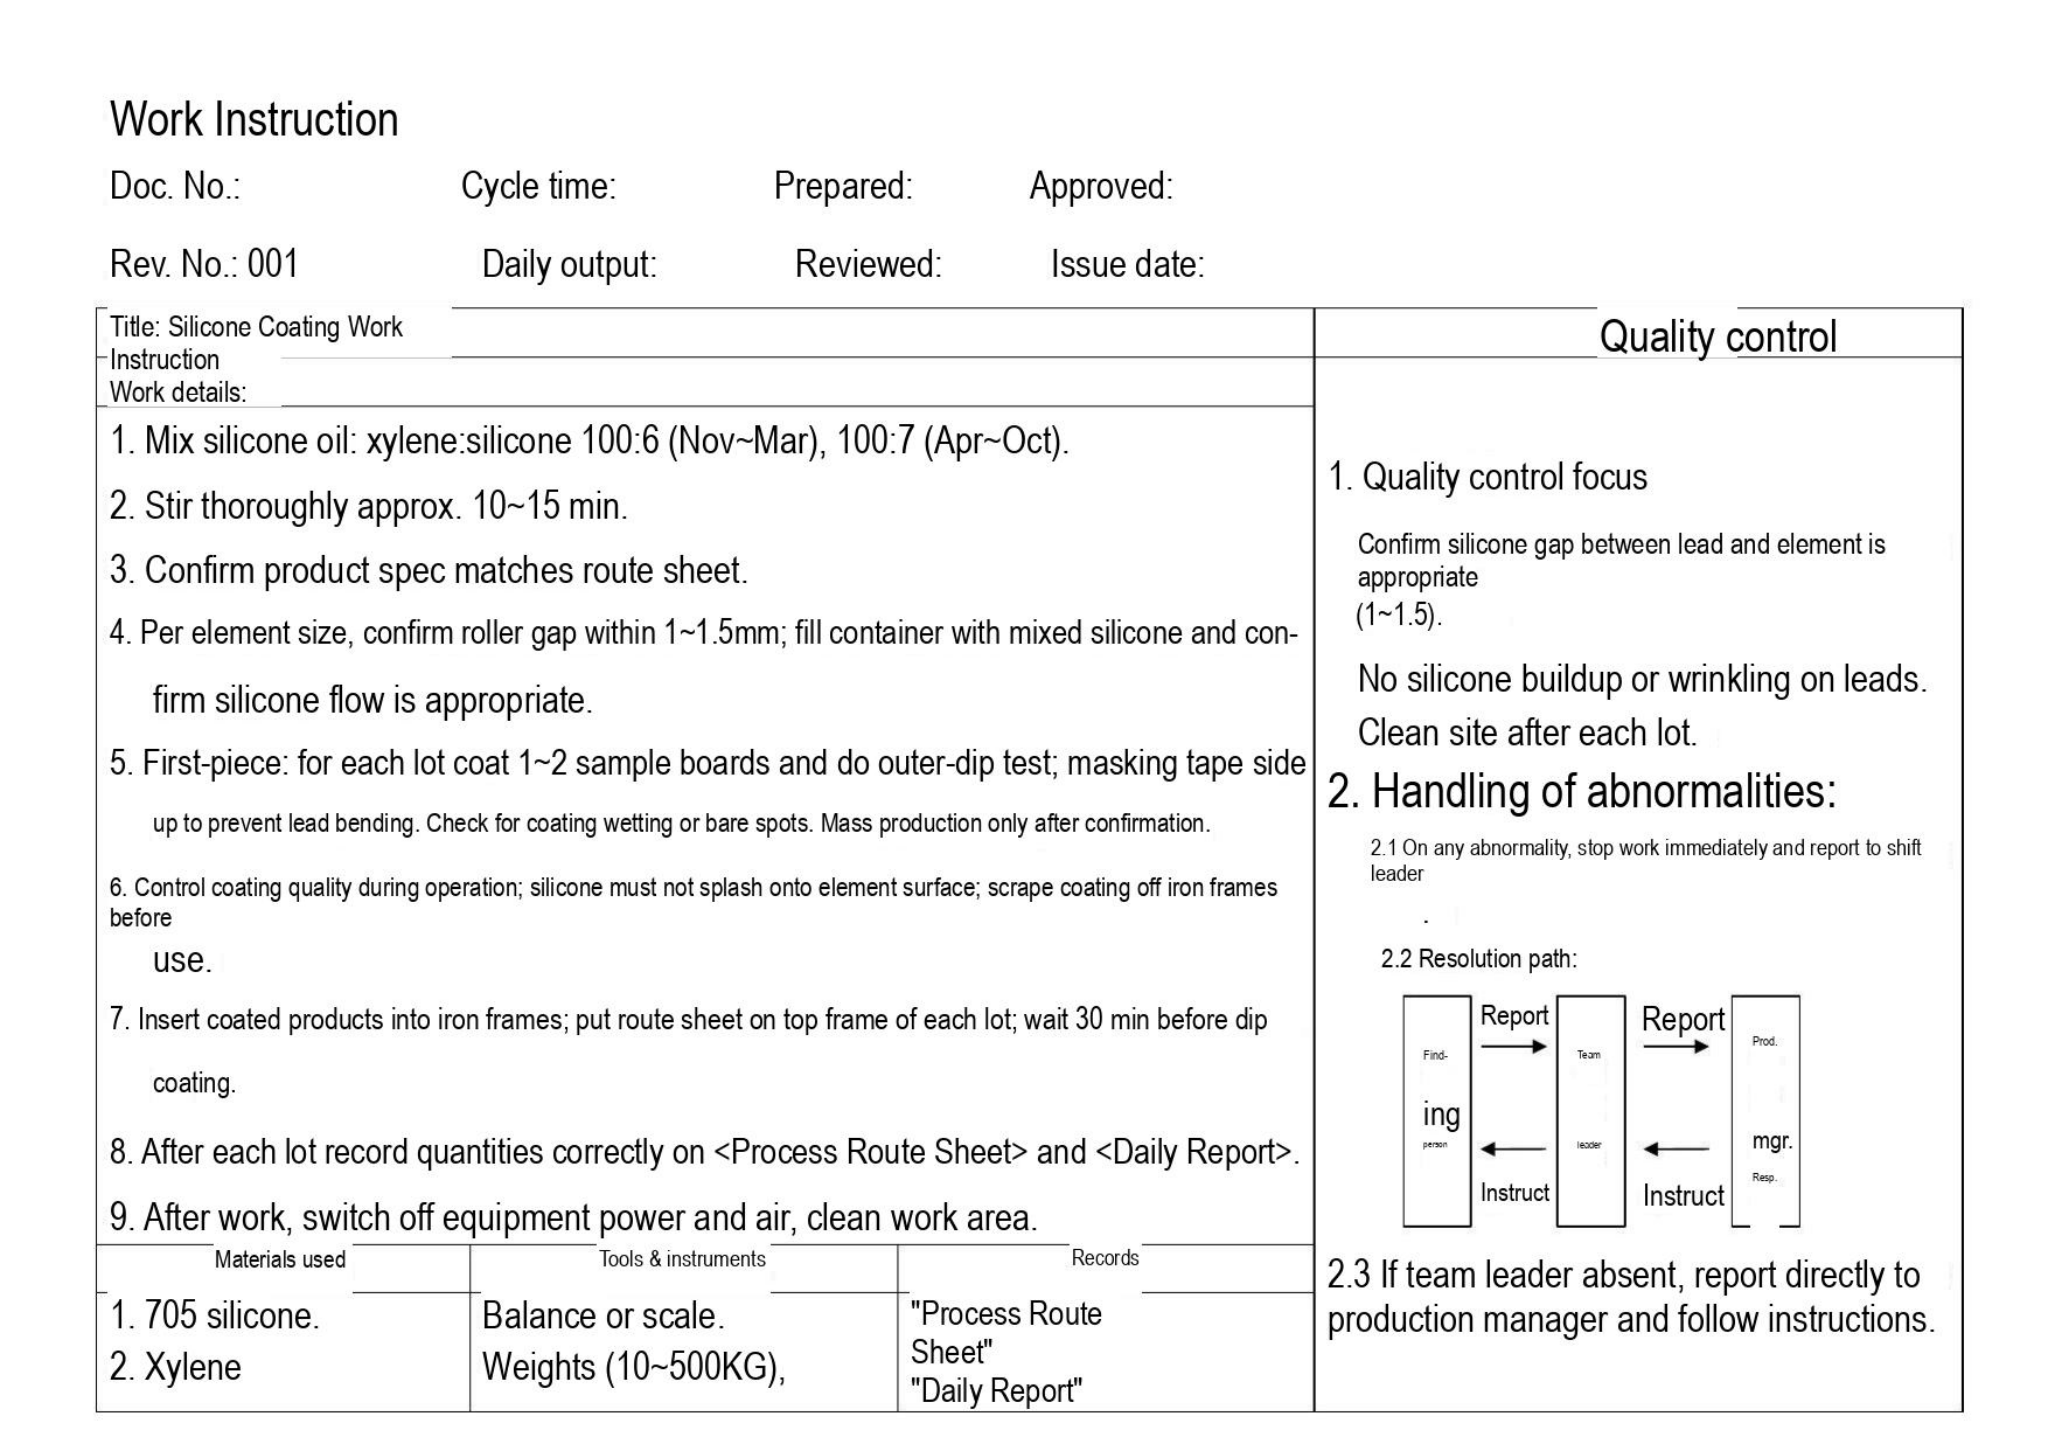Work Instruction

Doc. No.: Cycle time: Prepared: Approved:

Rev. No.: 001 Daily output: Reviewed: Issue date:

Title: Silicone Coating Work Instruction
Work details:

1. Mix silicone oil: xylene:silicone 100:6 (Nov~Mar), 100:7 (Apr~Oct).

2. Stir thoroughly approx. 10~15 min.

3. Confirm product spec matches route sheet.

4. Per element size, confirm roller gap within 1~1.5mm; fill container with mixed silicone and confirm silicone flow is appropriate.

5. First-piece: for each lot coat 1~2 sample boards and do outer-dip test; masking tape side up to prevent lead bending. Check for coating wetting or bare spots. Mass production only after confirmation.

6. Control coating quality during operation; silicone must not splash onto element surface; scrape coating off iron frames before use.

7. Insert coated products into iron frames; put route sheet on top frame of each lot; wait 30 min before dip coating.

8. After each lot record quantities correctly on <Process Route Sheet> and <Daily Report>.

9. After work, switch off equipment power and air, clean work area.

| Materials used | Tools & instruments | Records |
|---|---|---|
| 1. 705 silicone.<br>2. Xylene | Balance or scale.<br>Weights (10~500KG), | "Process Route Sheet"<br>"Daily Report" |

Quality control

1. Quality control focus

Confirm silicone gap between lead and element is appropriate (1~1.5).

No silicone buildup or wrinkling on leads.

Clean site after each lot.

2. Handling of abnormalities:

2.1 On any abnormality, stop work immediately and report to shift leader

2.2 Resolution path:

Finding person
Report →
← Instruct
Team leader
Report →
← Instruct
Prod. Resp. mgr.

2.3 If team leader absent, report directly to production manager and follow instructions.